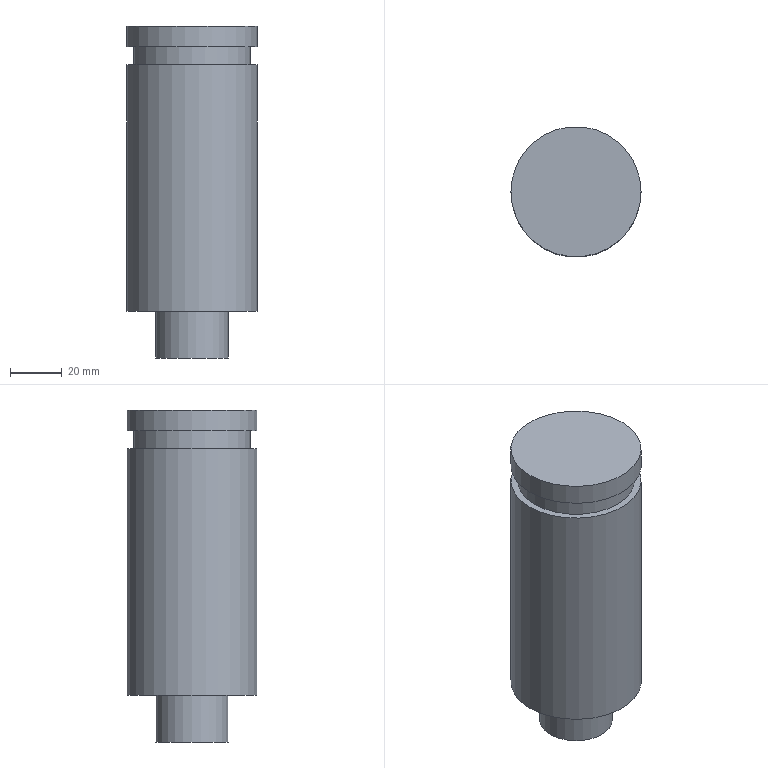Part | NX | features solid 2 | 1 solid | 9 faces | box 50.2 x 50.2 x 128 mm | volume 226078 mm3 | plane 5 | cylinder 4 | commonest cylinder face diameters 50.2 x2 28 x1 45 x1
STEP:
#1=CARTESIAN_POINT('',(180.1,580.,290.));
#2=VERTEX_POINT('',#1);
#3=CARTESIAN_POINT('',(155.,580.,290.));
#4=DIRECTION('',(0.,0.,1.));
#5=DIRECTION('',(1.,0.,0.));
#6=AXIS2_PLACEMENT_3D('',#3,#4,#5);
#7=CIRCLE('',#6,25.1);
#8=EDGE_CURVE('',#2,#2,#7,.F.);
#9=ORIENTED_EDGE('',*,*,#8,.T.);
#10=EDGE_LOOP('',(#9));
#11=FACE_BOUND('',#10,.T.);
#12=CARTESIAN_POINT('',(180.1,580.,282.));
#13=VERTEX_POINT('',#12);
#14=CARTESIAN_POINT('',(155.,580.,282.));
#15=DIRECTION('',(0.,0.,1.));
#16=DIRECTION('',(1.,0.,0.));
#17=AXIS2_PLACEMENT_3D('',#14,#15,#16);
#18=CIRCLE('',#17,25.1);
#19=EDGE_CURVE('',#13,#13,#18,.T.);
#20=ORIENTED_EDGE('',*,*,#19,.T.);
#21=EDGE_LOOP('',(#20));
#22=FACE_BOUND('',#21,.T.);
#23=CARTESIAN_POINT('',(155.,580.,290.));
#24=DIRECTION('',(0.,0.,-1.));
#25=DIRECTION('',(-1.,0.,0.));
#26=AXIS2_PLACEMENT_3D('',#23,#24,#25);
#27=CYLINDRICAL_SURFACE('',#26,25.1);
#28=ADVANCED_FACE('',(#11,#22),#27,.T.);
#29=ORIENTED_EDGE('',*,*,#8,.F.);
#30=EDGE_LOOP('',(#29));
#31=FACE_BOUND('',#30,.T.);
#32=CARTESIAN_POINT('',(155.,580.,290.));
#33=DIRECTION('',(0.,0.,-1.));
#34=DIRECTION('',(-1.,0.,0.));
#35=AXIS2_PLACEMENT_3D('',#32,#33,#34);
#36=PLANE('',#35);
#37=ADVANCED_FACE('',(#31),#36,.F.);
#38=CARTESIAN_POINT('',(177.5,580.,275.));
#39=VERTEX_POINT('',#38);
#40=CARTESIAN_POINT('',(155.,580.,275.));
#41=DIRECTION('',(0.,0.,1.));
#42=DIRECTION('',(1.,0.,0.));
#43=AXIS2_PLACEMENT_3D('',#40,#41,#42);
#44=CIRCLE('',#43,22.5);
#45=EDGE_CURVE('',#39,#39,#44,.F.);
#46=ORIENTED_EDGE('',*,*,#45,.F.);
#47=EDGE_LOOP('',(#46));
#48=FACE_BOUND('',#47,.T.);
#49=CARTESIAN_POINT('',(177.5,580.,282.));
#50=VERTEX_POINT('',#49);
#51=CARTESIAN_POINT('',(155.,580.,282.));
#52=DIRECTION('',(0.,0.,1.));
#53=DIRECTION('',(1.,0.,0.));
#54=AXIS2_PLACEMENT_3D('',#51,#52,#53);
#55=CIRCLE('',#54,22.5);
#56=EDGE_CURVE('',#50,#50,#55,.F.);
#57=ORIENTED_EDGE('',*,*,#56,.T.);
#58=EDGE_LOOP('',(#57));
#59=FACE_BOUND('',#58,.T.);
#60=CARTESIAN_POINT('',(155.,580.,278.5));
#61=DIRECTION('',(0.,0.,-1.));
#62=DIRECTION('',(-1.,0.,0.));
#63=AXIS2_PLACEMENT_3D('',#60,#61,#62);
#64=CYLINDRICAL_SURFACE('',#63,22.5);
#65=ADVANCED_FACE('',(#48,#59),#64,.T.);
#66=ORIENTED_EDGE('',*,*,#19,.F.);
#67=EDGE_LOOP('',(#66));
#68=FACE_BOUND('',#67,.T.);
#69=ORIENTED_EDGE('',*,*,#56,.F.);
#70=EDGE_LOOP('',(#69));
#71=FACE_BOUND('',#70,.T.);
#72=CARTESIAN_POINT('',(155.,580.,282.));
#73=DIRECTION('',(0.,0.,-1.));
#74=DIRECTION('',(-1.,0.,0.));
#75=AXIS2_PLACEMENT_3D('',#72,#73,#74);
#76=PLANE('',#75);
#77=ADVANCED_FACE('',(#68,#71),#76,.T.);
#78=CARTESIAN_POINT('',(180.1,580.,275.));
#79=VERTEX_POINT('',#78);
#80=CARTESIAN_POINT('',(155.,580.,275.));
#81=DIRECTION('',(0.,0.,1.));
#82=DIRECTION('',(1.,0.,0.));
#83=AXIS2_PLACEMENT_3D('',#80,#81,#82);
#84=CIRCLE('',#83,25.1);
#85=EDGE_CURVE('',#79,#79,#84,.T.);
#86=ORIENTED_EDGE('',*,*,#85,.T.);
#87=EDGE_LOOP('',(#86));
#88=FACE_BOUND('',#87,.T.);
#89=ORIENTED_EDGE('',*,*,#45,.T.);
#90=EDGE_LOOP('',(#89));
#91=FACE_BOUND('',#90,.T.);
#92=CARTESIAN_POINT('',(155.,580.,275.));
#93=DIRECTION('',(0.,0.,-1.));
#94=DIRECTION('',(-1.,0.,0.));
#95=AXIS2_PLACEMENT_3D('',#92,#93,#94);
#96=PLANE('',#95);
#97=ADVANCED_FACE('',(#88,#91),#96,.F.);
#98=ORIENTED_EDGE('',*,*,#85,.F.);
#99=EDGE_LOOP('',(#98));
#100=FACE_BOUND('',#99,.T.);
#101=CARTESIAN_POINT('',(180.1,580.,180.));
#102=VERTEX_POINT('',#101);
#103=CARTESIAN_POINT('',(155.,580.,180.));
#104=DIRECTION('',(0.,0.,1.));
#105=DIRECTION('',(1.,0.,0.));
#106=AXIS2_PLACEMENT_3D('',#103,#104,#105);
#107=CIRCLE('',#106,25.1);
#108=EDGE_CURVE('',#102,#102,#107,.F.);
#109=ORIENTED_EDGE('',*,*,#108,.F.);
#110=EDGE_LOOP('',(#109));
#111=FACE_BOUND('',#110,.T.);
#112=CARTESIAN_POINT('',(155.,580.,290.));
#113=DIRECTION('',(0.,0.,-1.));
#114=DIRECTION('',(-1.,0.,0.));
#115=AXIS2_PLACEMENT_3D('',#112,#113,#114);
#116=CYLINDRICAL_SURFACE('',#115,25.1);
#117=ADVANCED_FACE('',(#100,#111),#116,.T.);
#118=CARTESIAN_POINT('',(169.,580.,180.));
#119=VERTEX_POINT('',#118);
#120=CARTESIAN_POINT('',(155.,580.,180.));
#121=DIRECTION('',(0.,0.,1.));
#122=DIRECTION('',(1.,0.,0.));
#123=AXIS2_PLACEMENT_3D('',#120,#121,#122);
#124=CIRCLE('',#123,14.);
#125=EDGE_CURVE('',#119,#119,#124,.F.);
#126=ORIENTED_EDGE('',*,*,#125,.F.);
#127=EDGE_LOOP('',(#126));
#128=FACE_BOUND('',#127,.T.);
#129=ORIENTED_EDGE('',*,*,#108,.T.);
#130=EDGE_LOOP('',(#129));
#131=FACE_BOUND('',#130,.T.);
#132=CARTESIAN_POINT('',(155.,580.,180.));
#133=DIRECTION('',(0.,0.,-1.));
#134=DIRECTION('',(-1.,0.,0.));
#135=AXIS2_PLACEMENT_3D('',#132,#133,#134);
#136=PLANE('',#135);
#137=ADVANCED_FACE('',(#128,#131),#136,.T.);
#138=ORIENTED_EDGE('',*,*,#125,.T.);
#139=EDGE_LOOP('',(#138));
#140=FACE_BOUND('',#139,.T.);
#141=CARTESIAN_POINT('',(141.,580.,162.));
#142=VERTEX_POINT('',#141);
#143=CARTESIAN_POINT('',(155.,580.,162.));
#144=DIRECTION('',(0.,0.,-1.));
#145=DIRECTION('',(-1.,0.,0.));
#146=AXIS2_PLACEMENT_3D('',#143,#144,#145);
#147=CIRCLE('',#146,14.);
#148=EDGE_CURVE('',#142,#142,#147,.T.);
#149=ORIENTED_EDGE('',*,*,#148,.F.);
#150=EDGE_LOOP('',(#149));
#151=FACE_BOUND('',#150,.T.);
#152=CARTESIAN_POINT('',(155.,580.,169.5));
#153=DIRECTION('',(0.,0.,-1.));
#154=DIRECTION('',(-1.,0.,0.));
#155=AXIS2_PLACEMENT_3D('',#152,#153,#154);
#156=CYLINDRICAL_SURFACE('',#155,14.);
#157=ADVANCED_FACE('',(#140,#151),#156,.T.);
#158=ORIENTED_EDGE('',*,*,#148,.T.);
#159=EDGE_LOOP('',(#158));
#160=FACE_BOUND('',#159,.T.);
#161=CARTESIAN_POINT('',(-395.,150.,162.));
#162=DIRECTION('',(0.,0.,1.));
#163=DIRECTION('',(-1.,0.,0.));
#164=AXIS2_PLACEMENT_3D('',#161,#162,#163);
#165=PLANE('',#164);
#166=ADVANCED_FACE('',(#160),#165,.F.);
#167=CLOSED_SHELL('',(#28,#37,#65,#77,#97,#117,#137,#157,#166));
#168=MANIFOLD_SOLID_BREP('',#167);
#169=(LENGTH_UNIT()NAMED_UNIT(*)SI_UNIT(.MILLI.,.METRE.));
#170=UNCERTAINTY_MEASURE_WITH_UNIT(LENGTH_MEASURE(0.00001),#169,'','');
#171=(NAMED_UNIT(*)PLANE_ANGLE_UNIT()SI_UNIT($,.RADIAN.));
#172=(NAMED_UNIT(*)SI_UNIT($,.STERADIAN.)SOLID_ANGLE_UNIT());
#173=(GEOMETRIC_REPRESENTATION_CONTEXT(3)GLOBAL_UNCERTAINTY_ASSIGNED_CONTEXT((#170))GLOBAL_UNIT_ASSIGNED_CONTEXT((#169,#171,#172))REPRESENTATION_CONTEXT('',''));
#174=ADVANCED_BREP_SHAPE_REPRESENTATION('',(#168),#173);